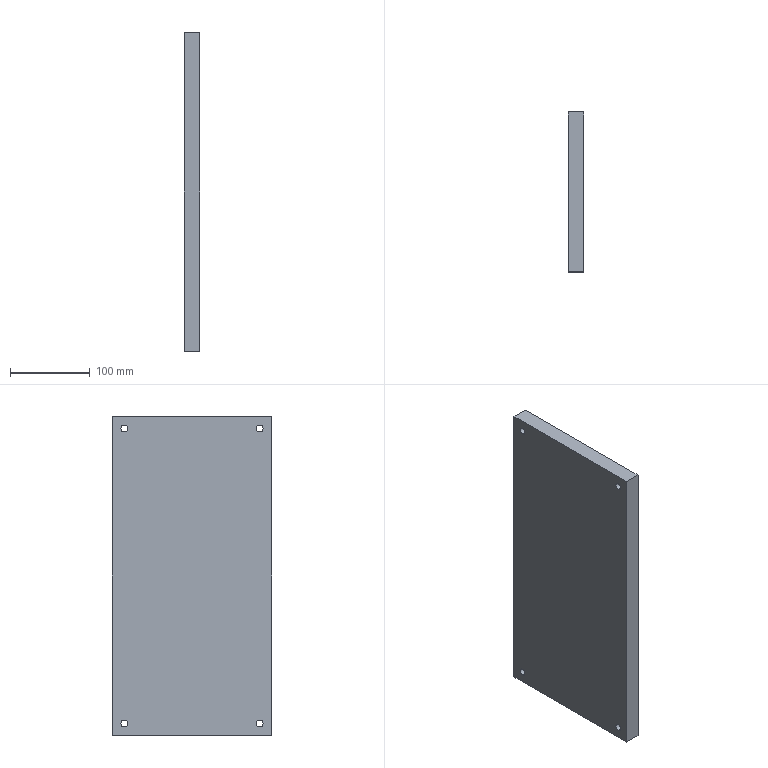Part | STEP file | A14-030-1 | 1 solid | 14 faces | box 20 x 200 x 400 mm | volume 1595460 mm3 | cylinder 8 | plane 6 | commonest cylinder face diameters 8.5 x8
STEP:
#1=CARTESIAN_POINT('',(0.,0.,0.));
#2=DIRECTION('',(0.,0.,1.));
#3=DIRECTION('',(1.,0.,0.));
#4=AXIS2_PLACEMENT_3D('',#1,#2,#3);
#5=CARTESIAN_POINT('',(-10.,85.,180.75));
#6=VERTEX_POINT('',#5);
#7=CARTESIAN_POINT('',(10.,85.,180.75));
#8=VERTEX_POINT('',#7);
#9=CARTESIAN_POINT('',(-10.,85.,180.75));
#10=DIRECTION('',(1.,0.,0.));
#11=VECTOR('',#10,1.);
#12=LINE('',#9,#11);
#13=CARTESIAN_POINT('',(-10.,85.,185.));
#14=DIRECTION('',(1.,0.,0.));
#15=DIRECTION('',(0.,0.,-1.));
#16=AXIS2_PLACEMENT_3D('',#13,#14,#15);
#17=CYLINDRICAL_SURFACE('',#16,4.25);
#18=CARTESIAN_POINT('',(6.283,0.));
#19=DIRECTION('',(0.,1.));
#20=VECTOR('',#19,1.);
#21=LINE('',#18,#20);
#22=(GEOMETRIC_REPRESENTATION_CONTEXT(2)PARAMETRIC_REPRESENTATION_CONTEXT()REPRESENTATION_CONTEXT('',''));
#23=DEFINITIONAL_REPRESENTATION('',(#21),#22);
#24=PCURVE('',#17,#23);
#25=CARTESIAN_POINT('',(-10.,85.,185.));
#26=DIRECTION('',(1.,0.,0.));
#27=DIRECTION('',(0.,0.,-1.));
#28=AXIS2_PLACEMENT_3D('',#25,#26,#27);
#29=CYLINDRICAL_SURFACE('',#28,4.25);
#30=CARTESIAN_POINT('',(0.,0.));
#31=DIRECTION('',(0.,1.));
#32=VECTOR('',#31,1.);
#33=LINE('',#30,#32);
#34=(GEOMETRIC_REPRESENTATION_CONTEXT(2)PARAMETRIC_REPRESENTATION_CONTEXT()REPRESENTATION_CONTEXT('',''));
#35=DEFINITIONAL_REPRESENTATION('',(#33),#34);
#36=PCURVE('',#29,#35);
#37=SURFACE_CURVE('',#12,(#24,#36),.PCURVE_S1.);
#38=EDGE_CURVE('',#6,#8,#37,.T.);
#39=ORIENTED_EDGE('',*,*,#38,.T.);
#40=CARTESIAN_POINT('',(10.,85.,189.25));
#41=VERTEX_POINT('',#40);
#42=CARTESIAN_POINT('',(10.,85.,185.));
#43=DIRECTION('',(1.,0.,0.));
#44=DIRECTION('',(0.,0.,-1.));
#45=AXIS2_PLACEMENT_3D('',#42,#43,#44);
#46=CIRCLE('',#45,4.25);
#47=CARTESIAN_POINT('',(0.,20.));
#48=DIRECTION('',(1.,0.));
#49=VECTOR('',#48,1.);
#50=LINE('',#47,#49);
#51=(GEOMETRIC_REPRESENTATION_CONTEXT(2)PARAMETRIC_REPRESENTATION_CONTEXT()REPRESENTATION_CONTEXT('',''));
#52=DEFINITIONAL_REPRESENTATION('',(#50),#51);
#53=PCURVE('',#17,#52);
#54=CARTESIAN_POINT('',(10.,0.,0.));
#55=DIRECTION('',(1.,0.,0.));
#56=DIRECTION('',(0.,0.,-1.));
#57=AXIS2_PLACEMENT_3D('',#54,#55,#56);
#58=PLANE('',#57);
#59=CARTESIAN_POINT('',(-185.,85.));
#60=DIRECTION('',(1.,0.));
#61=AXIS2_PLACEMENT_2D('',#59,#60);
#62=CIRCLE('',#61,4.25);
#63=(GEOMETRIC_REPRESENTATION_CONTEXT(2)PARAMETRIC_REPRESENTATION_CONTEXT()REPRESENTATION_CONTEXT('',''));
#64=DEFINITIONAL_REPRESENTATION('',(#62),#63);
#65=PCURVE('',#58,#64);
#66=SURFACE_CURVE('',#46,(#53,#65),.PCURVE_S1.);
#67=EDGE_CURVE('',#41,#8,#66,.T.);
#68=ORIENTED_EDGE('',*,*,#67,.F.);
#69=CARTESIAN_POINT('',(-10.,85.,189.25));
#70=VERTEX_POINT('',#69);
#71=CARTESIAN_POINT('',(-10.,85.,189.25));
#72=DIRECTION('',(1.,0.,0.));
#73=VECTOR('',#72,1.);
#74=LINE('',#71,#73);
#75=CARTESIAN_POINT('',(3.142,0.));
#76=DIRECTION('',(0.,1.));
#77=VECTOR('',#76,1.);
#78=LINE('',#75,#77);
#79=(GEOMETRIC_REPRESENTATION_CONTEXT(2)PARAMETRIC_REPRESENTATION_CONTEXT()REPRESENTATION_CONTEXT('',''));
#80=DEFINITIONAL_REPRESENTATION('',(#78),#79);
#81=PCURVE('',#17,#80);
#82=CARTESIAN_POINT('',(3.142,0.));
#83=DIRECTION('',(0.,1.));
#84=VECTOR('',#83,1.);
#85=LINE('',#82,#84);
#86=(GEOMETRIC_REPRESENTATION_CONTEXT(2)PARAMETRIC_REPRESENTATION_CONTEXT()REPRESENTATION_CONTEXT('',''));
#87=DEFINITIONAL_REPRESENTATION('',(#85),#86);
#88=PCURVE('',#29,#87);
#89=SURFACE_CURVE('',#74,(#81,#88),.PCURVE_S1.);
#90=EDGE_CURVE('',#70,#41,#89,.T.);
#91=ORIENTED_EDGE('',*,*,#90,.F.);
#92=CARTESIAN_POINT('',(-10.,85.,185.));
#93=DIRECTION('',(1.,0.,0.));
#94=DIRECTION('',(0.,0.,-1.));
#95=AXIS2_PLACEMENT_3D('',#92,#93,#94);
#96=CIRCLE('',#95,4.25);
#97=CARTESIAN_POINT('',(0.,0.));
#98=DIRECTION('',(1.,0.));
#99=VECTOR('',#98,1.);
#100=LINE('',#97,#99);
#101=(GEOMETRIC_REPRESENTATION_CONTEXT(2)PARAMETRIC_REPRESENTATION_CONTEXT()REPRESENTATION_CONTEXT('',''));
#102=DEFINITIONAL_REPRESENTATION('',(#100),#101);
#103=PCURVE('',#17,#102);
#104=CARTESIAN_POINT('',(-10.,0.,0.));
#105=DIRECTION('',(1.,0.,0.));
#106=DIRECTION('',(0.,0.,-1.));
#107=AXIS2_PLACEMENT_3D('',#104,#105,#106);
#108=PLANE('',#107);
#109=CARTESIAN_POINT('',(-185.,85.));
#110=DIRECTION('',(1.,0.));
#111=AXIS2_PLACEMENT_2D('',#109,#110);
#112=CIRCLE('',#111,4.25);
#113=(GEOMETRIC_REPRESENTATION_CONTEXT(2)PARAMETRIC_REPRESENTATION_CONTEXT()REPRESENTATION_CONTEXT('',''));
#114=DEFINITIONAL_REPRESENTATION('',(#112),#113);
#115=PCURVE('',#108,#114);
#116=SURFACE_CURVE('',#96,(#103,#115),.PCURVE_S1.);
#117=EDGE_CURVE('',#70,#6,#116,.T.);
#118=ORIENTED_EDGE('',*,*,#117,.T.);
#119=EDGE_LOOP('',(#39,#68,#91,#118));
#120=FACE_BOUND('',#119,.F.);
#121=ADVANCED_FACE('',(#120),#17,.F.);
#122=CARTESIAN_POINT('',(-10.,-85.,180.75));
#123=VERTEX_POINT('',#122);
#124=CARTESIAN_POINT('',(10.,-85.,180.75));
#125=VERTEX_POINT('',#124);
#126=CARTESIAN_POINT('',(-10.,-85.,180.75));
#127=DIRECTION('',(1.,0.,0.));
#128=VECTOR('',#127,1.);
#129=LINE('',#126,#128);
#130=CARTESIAN_POINT('',(-10.,-85.,185.));
#131=DIRECTION('',(1.,0.,0.));
#132=DIRECTION('',(0.,0.,-1.));
#133=AXIS2_PLACEMENT_3D('',#130,#131,#132);
#134=CYLINDRICAL_SURFACE('',#133,4.25);
#135=CARTESIAN_POINT('',(6.283,0.));
#136=DIRECTION('',(0.,1.));
#137=VECTOR('',#136,1.);
#138=LINE('',#135,#137);
#139=(GEOMETRIC_REPRESENTATION_CONTEXT(2)PARAMETRIC_REPRESENTATION_CONTEXT()REPRESENTATION_CONTEXT('',''));
#140=DEFINITIONAL_REPRESENTATION('',(#138),#139);
#141=PCURVE('',#134,#140);
#142=CARTESIAN_POINT('',(-10.,-85.,185.));
#143=DIRECTION('',(1.,0.,0.));
#144=DIRECTION('',(0.,0.,-1.));
#145=AXIS2_PLACEMENT_3D('',#142,#143,#144);
#146=CYLINDRICAL_SURFACE('',#145,4.25);
#147=CARTESIAN_POINT('',(0.,0.));
#148=DIRECTION('',(0.,1.));
#149=VECTOR('',#148,1.);
#150=LINE('',#147,#149);
#151=(GEOMETRIC_REPRESENTATION_CONTEXT(2)PARAMETRIC_REPRESENTATION_CONTEXT()REPRESENTATION_CONTEXT('',''));
#152=DEFINITIONAL_REPRESENTATION('',(#150),#151);
#153=PCURVE('',#146,#152);
#154=SURFACE_CURVE('',#129,(#141,#153),.PCURVE_S1.);
#155=EDGE_CURVE('',#123,#125,#154,.T.);
#156=ORIENTED_EDGE('',*,*,#155,.T.);
#157=CARTESIAN_POINT('',(10.,-85.,189.25));
#158=VERTEX_POINT('',#157);
#159=CARTESIAN_POINT('',(10.,-85.,185.));
#160=DIRECTION('',(1.,0.,0.));
#161=DIRECTION('',(0.,0.,-1.));
#162=AXIS2_PLACEMENT_3D('',#159,#160,#161);
#163=CIRCLE('',#162,4.25);
#164=CARTESIAN_POINT('',(0.,20.));
#165=DIRECTION('',(1.,0.));
#166=VECTOR('',#165,1.);
#167=LINE('',#164,#166);
#168=(GEOMETRIC_REPRESENTATION_CONTEXT(2)PARAMETRIC_REPRESENTATION_CONTEXT()REPRESENTATION_CONTEXT('',''));
#169=DEFINITIONAL_REPRESENTATION('',(#167),#168);
#170=PCURVE('',#134,#169);
#171=CARTESIAN_POINT('',(-185.,-85.));
#172=DIRECTION('',(1.,0.));
#173=AXIS2_PLACEMENT_2D('',#171,#172);
#174=CIRCLE('',#173,4.25);
#175=(GEOMETRIC_REPRESENTATION_CONTEXT(2)PARAMETRIC_REPRESENTATION_CONTEXT()REPRESENTATION_CONTEXT('',''));
#176=DEFINITIONAL_REPRESENTATION('',(#174),#175);
#177=PCURVE('',#58,#176);
#178=SURFACE_CURVE('',#163,(#170,#177),.PCURVE_S1.);
#179=EDGE_CURVE('',#158,#125,#178,.T.);
#180=ORIENTED_EDGE('',*,*,#179,.F.);
#181=CARTESIAN_POINT('',(-10.,-85.,189.25));
#182=VERTEX_POINT('',#181);
#183=CARTESIAN_POINT('',(-10.,-85.,189.25));
#184=DIRECTION('',(1.,0.,0.));
#185=VECTOR('',#184,1.);
#186=LINE('',#183,#185);
#187=CARTESIAN_POINT('',(3.142,0.));
#188=DIRECTION('',(0.,1.));
#189=VECTOR('',#188,1.);
#190=LINE('',#187,#189);
#191=(GEOMETRIC_REPRESENTATION_CONTEXT(2)PARAMETRIC_REPRESENTATION_CONTEXT()REPRESENTATION_CONTEXT('',''));
#192=DEFINITIONAL_REPRESENTATION('',(#190),#191);
#193=PCURVE('',#134,#192);
#194=CARTESIAN_POINT('',(3.142,0.));
#195=DIRECTION('',(0.,1.));
#196=VECTOR('',#195,1.);
#197=LINE('',#194,#196);
#198=(GEOMETRIC_REPRESENTATION_CONTEXT(2)PARAMETRIC_REPRESENTATION_CONTEXT()REPRESENTATION_CONTEXT('',''));
#199=DEFINITIONAL_REPRESENTATION('',(#197),#198);
#200=PCURVE('',#146,#199);
#201=SURFACE_CURVE('',#186,(#193,#200),.PCURVE_S1.);
#202=EDGE_CURVE('',#182,#158,#201,.T.);
#203=ORIENTED_EDGE('',*,*,#202,.F.);
#204=CARTESIAN_POINT('',(-10.,-85.,185.));
#205=DIRECTION('',(1.,0.,0.));
#206=DIRECTION('',(0.,0.,-1.));
#207=AXIS2_PLACEMENT_3D('',#204,#205,#206);
#208=CIRCLE('',#207,4.25);
#209=CARTESIAN_POINT('',(0.,0.));
#210=DIRECTION('',(1.,0.));
#211=VECTOR('',#210,1.);
#212=LINE('',#209,#211);
#213=(GEOMETRIC_REPRESENTATION_CONTEXT(2)PARAMETRIC_REPRESENTATION_CONTEXT()REPRESENTATION_CONTEXT('',''));
#214=DEFINITIONAL_REPRESENTATION('',(#212),#213);
#215=PCURVE('',#134,#214);
#216=CARTESIAN_POINT('',(-185.,-85.));
#217=DIRECTION('',(1.,0.));
#218=AXIS2_PLACEMENT_2D('',#216,#217);
#219=CIRCLE('',#218,4.25);
#220=(GEOMETRIC_REPRESENTATION_CONTEXT(2)PARAMETRIC_REPRESENTATION_CONTEXT()REPRESENTATION_CONTEXT('',''));
#221=DEFINITIONAL_REPRESENTATION('',(#219),#220);
#222=PCURVE('',#108,#221);
#223=SURFACE_CURVE('',#208,(#215,#222),.PCURVE_S1.);
#224=EDGE_CURVE('',#182,#123,#223,.T.);
#225=ORIENTED_EDGE('',*,*,#224,.T.);
#226=EDGE_LOOP('',(#156,#180,#203,#225));
#227=FACE_BOUND('',#226,.F.);
#228=ADVANCED_FACE('',(#227),#134,.F.);
#229=CARTESIAN_POINT('',(-10.,-85.,-189.25));
#230=VERTEX_POINT('',#229);
#231=CARTESIAN_POINT('',(10.,-85.,-189.25));
#232=VERTEX_POINT('',#231);
#233=CARTESIAN_POINT('',(-10.,-85.,-189.25));
#234=DIRECTION('',(1.,0.,0.));
#235=VECTOR('',#234,1.);
#236=LINE('',#233,#235);
#237=CARTESIAN_POINT('',(-10.,-85.,-185.));
#238=DIRECTION('',(1.,0.,0.));
#239=DIRECTION('',(0.,0.,-1.));
#240=AXIS2_PLACEMENT_3D('',#237,#238,#239);
#241=CYLINDRICAL_SURFACE('',#240,4.25);
#242=CARTESIAN_POINT('',(6.283,0.));
#243=DIRECTION('',(0.,1.));
#244=VECTOR('',#243,1.);
#245=LINE('',#242,#244);
#246=(GEOMETRIC_REPRESENTATION_CONTEXT(2)PARAMETRIC_REPRESENTATION_CONTEXT()REPRESENTATION_CONTEXT('',''));
#247=DEFINITIONAL_REPRESENTATION('',(#245),#246);
#248=PCURVE('',#241,#247);
#249=CARTESIAN_POINT('',(-10.,-85.,-185.));
#250=DIRECTION('',(1.,0.,0.));
#251=DIRECTION('',(0.,0.,-1.));
#252=AXIS2_PLACEMENT_3D('',#249,#250,#251);
#253=CYLINDRICAL_SURFACE('',#252,4.25);
#254=CARTESIAN_POINT('',(0.,0.));
#255=DIRECTION('',(0.,1.));
#256=VECTOR('',#255,1.);
#257=LINE('',#254,#256);
#258=(GEOMETRIC_REPRESENTATION_CONTEXT(2)PARAMETRIC_REPRESENTATION_CONTEXT()REPRESENTATION_CONTEXT('',''));
#259=DEFINITIONAL_REPRESENTATION('',(#257),#258);
#260=PCURVE('',#253,#259);
#261=SURFACE_CURVE('',#236,(#248,#260),.PCURVE_S1.);
#262=EDGE_CURVE('',#230,#232,#261,.T.);
#263=ORIENTED_EDGE('',*,*,#262,.T.);
#264=CARTESIAN_POINT('',(10.,-85.,-180.75));
#265=VERTEX_POINT('',#264);
#266=CARTESIAN_POINT('',(10.,-85.,-185.));
#267=DIRECTION('',(1.,0.,0.));
#268=DIRECTION('',(0.,0.,-1.));
#269=AXIS2_PLACEMENT_3D('',#266,#267,#268);
#270=CIRCLE('',#269,4.25);
#271=CARTESIAN_POINT('',(0.,20.));
#272=DIRECTION('',(1.,0.));
#273=VECTOR('',#272,1.);
#274=LINE('',#271,#273);
#275=(GEOMETRIC_REPRESENTATION_CONTEXT(2)PARAMETRIC_REPRESENTATION_CONTEXT()REPRESENTATION_CONTEXT('',''));
#276=DEFINITIONAL_REPRESENTATION('',(#274),#275);
#277=PCURVE('',#241,#276);
#278=CARTESIAN_POINT('',(185.,-85.));
#279=DIRECTION('',(1.,0.));
#280=AXIS2_PLACEMENT_2D('',#278,#279);
#281=CIRCLE('',#280,4.25);
#282=(GEOMETRIC_REPRESENTATION_CONTEXT(2)PARAMETRIC_REPRESENTATION_CONTEXT()REPRESENTATION_CONTEXT('',''));
#283=DEFINITIONAL_REPRESENTATION('',(#281),#282);
#284=PCURVE('',#58,#283);
#285=SURFACE_CURVE('',#270,(#277,#284),.PCURVE_S1.);
#286=EDGE_CURVE('',#265,#232,#285,.T.);
#287=ORIENTED_EDGE('',*,*,#286,.F.);
#288=CARTESIAN_POINT('',(-10.,-85.,-180.75));
#289=VERTEX_POINT('',#288);
#290=CARTESIAN_POINT('',(-10.,-85.,-180.75));
#291=DIRECTION('',(1.,0.,0.));
#292=VECTOR('',#291,1.);
#293=LINE('',#290,#292);
#294=CARTESIAN_POINT('',(3.142,0.));
#295=DIRECTION('',(0.,1.));
#296=VECTOR('',#295,1.);
#297=LINE('',#294,#296);
#298=(GEOMETRIC_REPRESENTATION_CONTEXT(2)PARAMETRIC_REPRESENTATION_CONTEXT()REPRESENTATION_CONTEXT('',''));
#299=DEFINITIONAL_REPRESENTATION('',(#297),#298);
#300=PCURVE('',#241,#299);
#301=CARTESIAN_POINT('',(3.142,0.));
#302=DIRECTION('',(0.,1.));
#303=VECTOR('',#302,1.);
#304=LINE('',#301,#303);
#305=(GEOMETRIC_REPRESENTATION_CONTEXT(2)PARAMETRIC_REPRESENTATION_CONTEXT()REPRESENTATION_CONTEXT('',''));
#306=DEFINITIONAL_REPRESENTATION('',(#304),#305);
#307=PCURVE('',#253,#306);
#308=SURFACE_CURVE('',#293,(#300,#307),.PCURVE_S1.);
#309=EDGE_CURVE('',#289,#265,#308,.T.);
#310=ORIENTED_EDGE('',*,*,#309,.F.);
#311=CARTESIAN_POINT('',(-10.,-85.,-185.));
#312=DIRECTION('',(1.,0.,0.));
#313=DIRECTION('',(0.,0.,-1.));
#314=AXIS2_PLACEMENT_3D('',#311,#312,#313);
#315=CIRCLE('',#314,4.25);
#316=CARTESIAN_POINT('',(0.,0.));
#317=DIRECTION('',(1.,0.));
#318=VECTOR('',#317,1.);
#319=LINE('',#316,#318);
#320=(GEOMETRIC_REPRESENTATION_CONTEXT(2)PARAMETRIC_REPRESENTATION_CONTEXT()REPRESENTATION_CONTEXT('',''));
#321=DEFINITIONAL_REPRESENTATION('',(#319),#320);
#322=PCURVE('',#241,#321);
#323=CARTESIAN_POINT('',(185.,-85.));
#324=DIRECTION('',(1.,0.));
#325=AXIS2_PLACEMENT_2D('',#323,#324);
#326=CIRCLE('',#325,4.25);
#327=(GEOMETRIC_REPRESENTATION_CONTEXT(2)PARAMETRIC_REPRESENTATION_CONTEXT()REPRESENTATION_CONTEXT('',''));
#328=DEFINITIONAL_REPRESENTATION('',(#326),#327);
#329=PCURVE('',#108,#328);
#330=SURFACE_CURVE('',#315,(#322,#329),.PCURVE_S1.);
#331=EDGE_CURVE('',#289,#230,#330,.T.);
#332=ORIENTED_EDGE('',*,*,#331,.T.);
#333=EDGE_LOOP('',(#263,#287,#310,#332));
#334=FACE_BOUND('',#333,.F.);
#335=ADVANCED_FACE('',(#334),#241,.F.);
#336=CARTESIAN_POINT('',(-10.,85.,-189.25));
#337=VERTEX_POINT('',#336);
#338=CARTESIAN_POINT('',(10.,85.,-189.25));
#339=VERTEX_POINT('',#338);
#340=CARTESIAN_POINT('',(-10.,85.,-189.25));
#341=DIRECTION('',(1.,0.,0.));
#342=VECTOR('',#341,1.);
#343=LINE('',#340,#342);
#344=CARTESIAN_POINT('',(-10.,85.,-185.));
#345=DIRECTION('',(1.,0.,0.));
#346=DIRECTION('',(0.,0.,-1.));
#347=AXIS2_PLACEMENT_3D('',#344,#345,#346);
#348=CYLINDRICAL_SURFACE('',#347,4.25);
#349=CARTESIAN_POINT('',(6.283,0.));
#350=DIRECTION('',(0.,1.));
#351=VECTOR('',#350,1.);
#352=LINE('',#349,#351);
#353=(GEOMETRIC_REPRESENTATION_CONTEXT(2)PARAMETRIC_REPRESENTATION_CONTEXT()REPRESENTATION_CONTEXT('',''));
#354=DEFINITIONAL_REPRESENTATION('',(#352),#353);
#355=PCURVE('',#348,#354);
#356=CARTESIAN_POINT('',(-10.,85.,-185.));
#357=DIRECTION('',(1.,0.,0.));
#358=DIRECTION('',(0.,0.,-1.));
#359=AXIS2_PLACEMENT_3D('',#356,#357,#358);
#360=CYLINDRICAL_SURFACE('',#359,4.25);
#361=CARTESIAN_POINT('',(0.,0.));
#362=DIRECTION('',(0.,1.));
#363=VECTOR('',#362,1.);
#364=LINE('',#361,#363);
#365=(GEOMETRIC_REPRESENTATION_CONTEXT(2)PARAMETRIC_REPRESENTATION_CONTEXT()REPRESENTATION_CONTEXT('',''));
#366=DEFINITIONAL_REPRESENTATION('',(#364),#365);
#367=PCURVE('',#360,#366);
#368=SURFACE_CURVE('',#343,(#355,#367),.PCURVE_S1.);
#369=EDGE_CURVE('',#337,#339,#368,.T.);
#370=ORIENTED_EDGE('',*,*,#369,.T.);
#371=CARTESIAN_POINT('',(10.,85.,-180.75));
#372=VERTEX_POINT('',#371);
#373=CARTESIAN_POINT('',(10.,85.,-185.));
#374=DIRECTION('',(1.,0.,0.));
#375=DIRECTION('',(0.,0.,-1.));
#376=AXIS2_PLACEMENT_3D('',#373,#374,#375);
#377=CIRCLE('',#376,4.25);
#378=CARTESIAN_POINT('',(0.,20.));
#379=DIRECTION('',(1.,0.));
#380=VECTOR('',#379,1.);
#381=LINE('',#378,#380);
#382=(GEOMETRIC_REPRESENTATION_CONTEXT(2)PARAMETRIC_REPRESENTATION_CONTEXT()REPRESENTATION_CONTEXT('',''));
#383=DEFINITIONAL_REPRESENTATION('',(#381),#382);
#384=PCURVE('',#348,#383);
#385=CARTESIAN_POINT('',(185.,85.));
#386=DIRECTION('',(1.,0.));
#387=AXIS2_PLACEMENT_2D('',#385,#386);
#388=CIRCLE('',#387,4.25);
#389=(GEOMETRIC_REPRESENTATION_CONTEXT(2)PARAMETRIC_REPRESENTATION_CONTEXT()REPRESENTATION_CONTEXT('',''));
#390=DEFINITIONAL_REPRESENTATION('',(#388),#389);
#391=PCURVE('',#58,#390);
#392=SURFACE_CURVE('',#377,(#384,#391),.PCURVE_S1.);
#393=EDGE_CURVE('',#372,#339,#392,.T.);
#394=ORIENTED_EDGE('',*,*,#393,.F.);
#395=CARTESIAN_POINT('',(-10.,85.,-180.75));
#396=VERTEX_POINT('',#395);
#397=CARTESIAN_POINT('',(-10.,85.,-180.75));
#398=DIRECTION('',(1.,0.,0.));
#399=VECTOR('',#398,1.);
#400=LINE('',#397,#399);
#401=CARTESIAN_POINT('',(3.142,0.));
#402=DIRECTION('',(0.,1.));
#403=VECTOR('',#402,1.);
#404=LINE('',#401,#403);
#405=(GEOMETRIC_REPRESENTATION_CONTEXT(2)PARAMETRIC_REPRESENTATION_CONTEXT()REPRESENTATION_CONTEXT('',''));
#406=DEFINITIONAL_REPRESENTATION('',(#404),#405);
#407=PCURVE('',#348,#406);
#408=CARTESIAN_POINT('',(3.142,0.));
#409=DIRECTION('',(0.,1.));
#410=VECTOR('',#409,1.);
#411=LINE('',#408,#410);
#412=(GEOMETRIC_REPRESENTATION_CONTEXT(2)PARAMETRIC_REPRESENTATION_CONTEXT()REPRESENTATION_CONTEXT('',''));
#413=DEFINITIONAL_REPRESENTATION('',(#411),#412);
#414=PCURVE('',#360,#413);
#415=SURFACE_CURVE('',#400,(#407,#414),.PCURVE_S1.);
#416=EDGE_CURVE('',#396,#372,#415,.T.);
#417=ORIENTED_EDGE('',*,*,#416,.F.);
#418=CARTESIAN_POINT('',(-10.,85.,-185.));
#419=DIRECTION('',(1.,0.,0.));
#420=DIRECTION('',(0.,0.,-1.));
#421=AXIS2_PLACEMENT_3D('',#418,#419,#420);
#422=CIRCLE('',#421,4.25);
#423=CARTESIAN_POINT('',(0.,0.));
#424=DIRECTION('',(1.,0.));
#425=VECTOR('',#424,1.);
#426=LINE('',#423,#425);
#427=(GEOMETRIC_REPRESENTATION_CONTEXT(2)PARAMETRIC_REPRESENTATION_CONTEXT()REPRESENTATION_CONTEXT('',''));
#428=DEFINITIONAL_REPRESENTATION('',(#426),#427);
#429=PCURVE('',#348,#428);
#430=CARTESIAN_POINT('',(185.,85.));
#431=DIRECTION('',(1.,0.));
#432=AXIS2_PLACEMENT_2D('',#430,#431);
#433=CIRCLE('',#432,4.25);
#434=(GEOMETRIC_REPRESENTATION_CONTEXT(2)PARAMETRIC_REPRESENTATION_CONTEXT()REPRESENTATION_CONTEXT('',''));
#435=DEFINITIONAL_REPRESENTATION('',(#433),#434);
#436=PCURVE('',#108,#435);
#437=SURFACE_CURVE('',#422,(#429,#436),.PCURVE_S1.);
#438=EDGE_CURVE('',#396,#337,#437,.T.);
#439=ORIENTED_EDGE('',*,*,#438,.T.);
#440=EDGE_LOOP('',(#370,#394,#417,#439));
#441=FACE_BOUND('',#440,.F.);
#442=ADVANCED_FACE('',(#441),#348,.F.);
#443=CARTESIAN_POINT('',(-10.,-100.,-200.));
#444=VERTEX_POINT('',#443);
#445=CARTESIAN_POINT('',(-10.,100.,-200.));
#446=VERTEX_POINT('',#445);
#447=CARTESIAN_POINT('',(-10.,100.,-200.));
#448=DIRECTION('',(0.,1.,0.));
#449=VECTOR('',#448,1.);
#450=LINE('',#447,#449);
#451=CARTESIAN_POINT('',(10.,100.,-200.));
#452=DIRECTION('',(0.,0.,1.));
#453=DIRECTION('',(0.,-1.,0.));
#454=AXIS2_PLACEMENT_3D('',#451,#452,#453);
#455=PLANE('',#454);
#456=CARTESIAN_POINT('',(0.,-20.));
#457=DIRECTION('',(-1.,0.));
#458=VECTOR('',#457,1.);
#459=LINE('',#456,#458);
#460=(GEOMETRIC_REPRESENTATION_CONTEXT(2)PARAMETRIC_REPRESENTATION_CONTEXT()REPRESENTATION_CONTEXT('',''));
#461=DEFINITIONAL_REPRESENTATION('',(#459),#460);
#462=PCURVE('',#455,#461);
#463=CARTESIAN_POINT('',(200.,100.));
#464=DIRECTION('',(0.,1.));
#465=VECTOR('',#464,1.);
#466=LINE('',#463,#465);
#467=(GEOMETRIC_REPRESENTATION_CONTEXT(2)PARAMETRIC_REPRESENTATION_CONTEXT()REPRESENTATION_CONTEXT('',''));
#468=DEFINITIONAL_REPRESENTATION('',(#466),#467);
#469=PCURVE('',#108,#468);
#470=SURFACE_CURVE('',#450,(#462,#469),.PCURVE_S1.);
#471=EDGE_CURVE('',#444,#446,#470,.T.);
#472=ORIENTED_EDGE('',*,*,#471,.T.);
#473=CARTESIAN_POINT('',(10.,100.,-200.));
#474=VERTEX_POINT('',#473);
#475=CARTESIAN_POINT('',(10.,100.,-200.));
#476=DIRECTION('',(-1.,0.,0.));
#477=VECTOR('',#476,1.);
#478=LINE('',#475,#477);
#479=CARTESIAN_POINT('',(0.,0.));
#480=DIRECTION('',(0.,-1.));
#481=VECTOR('',#480,1.);
#482=LINE('',#479,#481);
#483=(GEOMETRIC_REPRESENTATION_CONTEXT(2)PARAMETRIC_REPRESENTATION_CONTEXT()REPRESENTATION_CONTEXT('',''));
#484=DEFINITIONAL_REPRESENTATION('',(#482),#483);
#485=PCURVE('',#455,#484);
#486=CARTESIAN_POINT('',(10.,100.,200.));
#487=DIRECTION('',(0.,-1.,0.));
#488=DIRECTION('',(0.,0.,-1.));
#489=AXIS2_PLACEMENT_3D('',#486,#487,#488);
#490=PLANE('',#489);
#491=CARTESIAN_POINT('',(400.,0.));
#492=DIRECTION('',(0.,-1.));
#493=VECTOR('',#492,1.);
#494=LINE('',#491,#493);
#495=(GEOMETRIC_REPRESENTATION_CONTEXT(2)PARAMETRIC_REPRESENTATION_CONTEXT()REPRESENTATION_CONTEXT('',''));
#496=DEFINITIONAL_REPRESENTATION('',(#494),#495);
#497=PCURVE('',#490,#496);
#498=SURFACE_CURVE('',#478,(#485,#497),.PCURVE_S1.);
#499=EDGE_CURVE('',#474,#446,#498,.T.);
#500=ORIENTED_EDGE('',*,*,#499,.F.);
#501=CARTESIAN_POINT('',(10.,-100.,-200.));
#502=VERTEX_POINT('',#501);
#503=CARTESIAN_POINT('',(10.,100.,-200.));
#504=DIRECTION('',(0.,1.,0.));
#505=VECTOR('',#504,1.);
#506=LINE('',#503,#505);
#507=CARTESIAN_POINT('',(0.,0.));
#508=DIRECTION('',(-1.,0.));
#509=VECTOR('',#508,1.);
#510=LINE('',#507,#509);
#511=(GEOMETRIC_REPRESENTATION_CONTEXT(2)PARAMETRIC_REPRESENTATION_CONTEXT()REPRESENTATION_CONTEXT('',''));
#512=DEFINITIONAL_REPRESENTATION('',(#510),#511);
#513=PCURVE('',#455,#512);
#514=CARTESIAN_POINT('',(200.,100.));
#515=DIRECTION('',(0.,1.));
#516=VECTOR('',#515,1.);
#517=LINE('',#514,#516);
#518=(GEOMETRIC_REPRESENTATION_CONTEXT(2)PARAMETRIC_REPRESENTATION_CONTEXT()REPRESENTATION_CONTEXT('',''));
#519=DEFINITIONAL_REPRESENTATION('',(#517),#518);
#520=PCURVE('',#58,#519);
#521=SURFACE_CURVE('',#506,(#513,#520),.PCURVE_S1.);
#522=EDGE_CURVE('',#502,#474,#521,.T.);
#523=ORIENTED_EDGE('',*,*,#522,.F.);
#524=CARTESIAN_POINT('',(10.,-100.,-200.));
#525=DIRECTION('',(-1.,0.,0.));
#526=VECTOR('',#525,1.);
#527=LINE('',#524,#526);
#528=CARTESIAN_POINT('',(200.,0.));
#529=DIRECTION('',(0.,-1.));
#530=VECTOR('',#529,1.);
#531=LINE('',#528,#530);
#532=(GEOMETRIC_REPRESENTATION_CONTEXT(2)PARAMETRIC_REPRESENTATION_CONTEXT()REPRESENTATION_CONTEXT('',''));
#533=DEFINITIONAL_REPRESENTATION('',(#531),#532);
#534=PCURVE('',#455,#533);
#535=CARTESIAN_POINT('',(10.,-100.,200.));
#536=DIRECTION('',(0.,1.,0.));
#537=DIRECTION('',(0.,0.,1.));
#538=AXIS2_PLACEMENT_3D('',#535,#536,#537);
#539=PLANE('',#538);
#540=CARTESIAN_POINT('',(-400.,0.));
#541=DIRECTION('',(0.,-1.));
#542=VECTOR('',#541,1.);
#543=LINE('',#540,#542);
#544=(GEOMETRIC_REPRESENTATION_CONTEXT(2)PARAMETRIC_REPRESENTATION_CONTEXT()REPRESENTATION_CONTEXT('',''));
#545=DEFINITIONAL_REPRESENTATION('',(#543),#544);
#546=PCURVE('',#539,#545);
#547=SURFACE_CURVE('',#527,(#534,#546),.PCURVE_S1.);
#548=EDGE_CURVE('',#502,#444,#547,.T.);
#549=ORIENTED_EDGE('',*,*,#548,.T.);
#550=EDGE_LOOP('',(#472,#500,#523,#549));
#551=FACE_BOUND('',#550,.T.);
#552=ADVANCED_FACE('',(#551),#455,.F.);
#553=CARTESIAN_POINT('',(-10.,100.,200.));
#554=VERTEX_POINT('',#553);
#555=CARTESIAN_POINT('',(-10.,100.,200.));
#556=DIRECTION('',(0.,0.,1.));
#557=VECTOR('',#556,1.);
#558=LINE('',#555,#557);
#559=CARTESIAN_POINT('',(0.,-20.));
#560=DIRECTION('',(-1.,0.));
#561=VECTOR('',#560,1.);
#562=LINE('',#559,#561);
#563=(GEOMETRIC_REPRESENTATION_CONTEXT(2)PARAMETRIC_REPRESENTATION_CONTEXT()REPRESENTATION_CONTEXT('',''));
#564=DEFINITIONAL_REPRESENTATION('',(#562),#563);
#565=PCURVE('',#490,#564);
#566=CARTESIAN_POINT('',(-200.,100.));
#567=DIRECTION('',(-1.,0.));
#568=VECTOR('',#567,1.);
#569=LINE('',#566,#568);
#570=(GEOMETRIC_REPRESENTATION_CONTEXT(2)PARAMETRIC_REPRESENTATION_CONTEXT()REPRESENTATION_CONTEXT('',''));
#571=DEFINITIONAL_REPRESENTATION('',(#569),#570);
#572=PCURVE('',#108,#571);
#573=SURFACE_CURVE('',#558,(#565,#572),.PCURVE_S1.);
#574=EDGE_CURVE('',#446,#554,#573,.T.);
#575=ORIENTED_EDGE('',*,*,#574,.T.);
#576=CARTESIAN_POINT('',(10.,100.,200.));
#577=VERTEX_POINT('',#576);
#578=CARTESIAN_POINT('',(10.,100.,200.));
#579=DIRECTION('',(-1.,0.,0.));
#580=VECTOR('',#579,1.);
#581=LINE('',#578,#580);
#582=CARTESIAN_POINT('',(0.,0.));
#583=DIRECTION('',(0.,-1.));
#584=VECTOR('',#583,1.);
#585=LINE('',#582,#584);
#586=(GEOMETRIC_REPRESENTATION_CONTEXT(2)PARAMETRIC_REPRESENTATION_CONTEXT()REPRESENTATION_CONTEXT('',''));
#587=DEFINITIONAL_REPRESENTATION('',(#585),#586);
#588=PCURVE('',#490,#587);
#589=CARTESIAN_POINT('',(10.,100.,200.));
#590=DIRECTION('',(0.,0.,-1.));
#591=DIRECTION('',(0.,1.,0.));
#592=AXIS2_PLACEMENT_3D('',#589,#590,#591);
#593=PLANE('',#592);
#594=CARTESIAN_POINT('',(0.,0.));
#595=DIRECTION('',(0.,-1.));
#596=VECTOR('',#595,1.);
#597=LINE('',#594,#596);
#598=(GEOMETRIC_REPRESENTATION_CONTEXT(2)PARAMETRIC_REPRESENTATION_CONTEXT()REPRESENTATION_CONTEXT('',''));
#599=DEFINITIONAL_REPRESENTATION('',(#597),#598);
#600=PCURVE('',#593,#599);
#601=SURFACE_CURVE('',#581,(#588,#600),.PCURVE_S1.);
#602=EDGE_CURVE('',#577,#554,#601,.T.);
#603=ORIENTED_EDGE('',*,*,#602,.F.);
#604=CARTESIAN_POINT('',(10.,100.,200.));
#605=DIRECTION('',(0.,0.,1.));
#606=VECTOR('',#605,1.);
#607=LINE('',#604,#606);
#608=CARTESIAN_POINT('',(0.,0.));
#609=DIRECTION('',(-1.,0.));
#610=VECTOR('',#609,1.);
#611=LINE('',#608,#610);
#612=(GEOMETRIC_REPRESENTATION_CONTEXT(2)PARAMETRIC_REPRESENTATION_CONTEXT()REPRESENTATION_CONTEXT('',''));
#613=DEFINITIONAL_REPRESENTATION('',(#611),#612);
#614=PCURVE('',#490,#613);
#615=CARTESIAN_POINT('',(-200.,100.));
#616=DIRECTION('',(-1.,0.));
#617=VECTOR('',#616,1.);
#618=LINE('',#615,#617);
#619=(GEOMETRIC_REPRESENTATION_CONTEXT(2)PARAMETRIC_REPRESENTATION_CONTEXT()REPRESENTATION_CONTEXT('',''));
#620=DEFINITIONAL_REPRESENTATION('',(#618),#619);
#621=PCURVE('',#58,#620);
#622=SURFACE_CURVE('',#607,(#614,#621),.PCURVE_S1.);
#623=EDGE_CURVE('',#474,#577,#622,.T.);
#624=ORIENTED_EDGE('',*,*,#623,.F.);
#625=ORIENTED_EDGE('',*,*,#499,.T.);
#626=EDGE_LOOP('',(#575,#603,#624,#625));
#627=FACE_BOUND('',#626,.T.);
#628=ADVANCED_FACE('',(#627),#490,.F.);
#629=CARTESIAN_POINT('',(-10.,-100.,200.));
#630=VERTEX_POINT('',#629);
#631=CARTESIAN_POINT('',(-10.,100.,200.));
#632=DIRECTION('',(0.,-1.,0.));
#633=VECTOR('',#632,1.);
#634=LINE('',#631,#633);
#635=CARTESIAN_POINT('',(0.,-20.));
#636=DIRECTION('',(-1.,0.));
#637=VECTOR('',#636,1.);
#638=LINE('',#635,#637);
#639=(GEOMETRIC_REPRESENTATION_CONTEXT(2)PARAMETRIC_REPRESENTATION_CONTEXT()REPRESENTATION_CONTEXT('',''));
#640=DEFINITIONAL_REPRESENTATION('',(#638),#639);
#641=PCURVE('',#593,#640);
#642=CARTESIAN_POINT('',(-200.,100.));
#643=DIRECTION('',(0.,-1.));
#644=VECTOR('',#643,1.);
#645=LINE('',#642,#644);
#646=(GEOMETRIC_REPRESENTATION_CONTEXT(2)PARAMETRIC_REPRESENTATION_CONTEXT()REPRESENTATION_CONTEXT('',''));
#647=DEFINITIONAL_REPRESENTATION('',(#645),#646);
#648=PCURVE('',#108,#647);
#649=SURFACE_CURVE('',#634,(#641,#648),.PCURVE_S1.);
#650=EDGE_CURVE('',#554,#630,#649,.T.);
#651=ORIENTED_EDGE('',*,*,#650,.T.);
#652=CARTESIAN_POINT('',(10.,-100.,200.));
#653=VERTEX_POINT('',#652);
#654=CARTESIAN_POINT('',(10.,-100.,200.));
#655=DIRECTION('',(-1.,0.,0.));
#656=VECTOR('',#655,1.);
#657=LINE('',#654,#656);
#658=CARTESIAN_POINT('',(-200.,0.));
#659=DIRECTION('',(0.,-1.));
#660=VECTOR('',#659,1.);
#661=LINE('',#658,#660);
#662=(GEOMETRIC_REPRESENTATION_CONTEXT(2)PARAMETRIC_REPRESENTATION_CONTEXT()REPRESENTATION_CONTEXT('',''));
#663=DEFINITIONAL_REPRESENTATION('',(#661),#662);
#664=PCURVE('',#593,#663);
#665=CARTESIAN_POINT('',(0.,0.));
#666=DIRECTION('',(0.,-1.));
#667=VECTOR('',#666,1.);
#668=LINE('',#665,#667);
#669=(GEOMETRIC_REPRESENTATION_CONTEXT(2)PARAMETRIC_REPRESENTATION_CONTEXT()REPRESENTATION_CONTEXT('',''));
#670=DEFINITIONAL_REPRESENTATION('',(#668),#669);
#671=PCURVE('',#539,#670);
#672=SURFACE_CURVE('',#657,(#664,#671),.PCURVE_S1.);
#673=EDGE_CURVE('',#653,#630,#672,.T.);
#674=ORIENTED_EDGE('',*,*,#673,.F.);
#675=CARTESIAN_POINT('',(10.,100.,200.));
#676=DIRECTION('',(0.,-1.,0.));
#677=VECTOR('',#676,1.);
#678=LINE('',#675,#677);
#679=CARTESIAN_POINT('',(0.,0.));
#680=DIRECTION('',(-1.,0.));
#681=VECTOR('',#680,1.);
#682=LINE('',#679,#681);
#683=(GEOMETRIC_REPRESENTATION_CONTEXT(2)PARAMETRIC_REPRESENTATION_CONTEXT()REPRESENTATION_CONTEXT('',''));
#684=DEFINITIONAL_REPRESENTATION('',(#682),#683);
#685=PCURVE('',#593,#684);
#686=CARTESIAN_POINT('',(-200.,100.));
#687=DIRECTION('',(0.,-1.));
#688=VECTOR('',#687,1.);
#689=LINE('',#686,#688);
#690=(GEOMETRIC_REPRESENTATION_CONTEXT(2)PARAMETRIC_REPRESENTATION_CONTEXT()REPRESENTATION_CONTEXT('',''));
#691=DEFINITIONAL_REPRESENTATION('',(#689),#690);
#692=PCURVE('',#58,#691);
#693=SURFACE_CURVE('',#678,(#685,#692),.PCURVE_S1.);
#694=EDGE_CURVE('',#577,#653,#693,.T.);
#695=ORIENTED_EDGE('',*,*,#694,.F.);
#696=ORIENTED_EDGE('',*,*,#602,.T.);
#697=EDGE_LOOP('',(#651,#674,#695,#696));
#698=FACE_BOUND('',#697,.T.);
#699=ADVANCED_FACE('',(#698),#593,.F.);
#700=CARTESIAN_POINT('',(-10.,-100.,200.));
#701=DIRECTION('',(0.,0.,-1.));
#702=VECTOR('',#701,1.);
#703=LINE('',#700,#702);
#704=CARTESIAN_POINT('',(0.,-20.));
#705=DIRECTION('',(-1.,0.));
#706=VECTOR('',#705,1.);
#707=LINE('',#704,#706);
#708=(GEOMETRIC_REPRESENTATION_CONTEXT(2)PARAMETRIC_REPRESENTATION_CONTEXT()REPRESENTATION_CONTEXT('',''));
#709=DEFINITIONAL_REPRESENTATION('',(#707),#708);
#710=PCURVE('',#539,#709);
#711=CARTESIAN_POINT('',(-200.,-100.));
#712=DIRECTION('',(1.,0.));
#713=VECTOR('',#712,1.);
#714=LINE('',#711,#713);
#715=(GEOMETRIC_REPRESENTATION_CONTEXT(2)PARAMETRIC_REPRESENTATION_CONTEXT()REPRESENTATION_CONTEXT('',''));
#716=DEFINITIONAL_REPRESENTATION('',(#714),#715);
#717=PCURVE('',#108,#716);
#718=SURFACE_CURVE('',#703,(#710,#717),.PCURVE_S1.);
#719=EDGE_CURVE('',#630,#444,#718,.T.);
#720=ORIENTED_EDGE('',*,*,#719,.T.);
#721=ORIENTED_EDGE('',*,*,#548,.F.);
#722=CARTESIAN_POINT('',(10.,-100.,200.));
#723=DIRECTION('',(0.,0.,-1.));
#724=VECTOR('',#723,1.);
#725=LINE('',#722,#724);
#726=CARTESIAN_POINT('',(0.,0.));
#727=DIRECTION('',(-1.,0.));
#728=VECTOR('',#727,1.);
#729=LINE('',#726,#728);
#730=(GEOMETRIC_REPRESENTATION_CONTEXT(2)PARAMETRIC_REPRESENTATION_CONTEXT()REPRESENTATION_CONTEXT('',''));
#731=DEFINITIONAL_REPRESENTATION('',(#729),#730);
#732=PCURVE('',#539,#731);
#733=CARTESIAN_POINT('',(-200.,-100.));
#734=DIRECTION('',(1.,0.));
#735=VECTOR('',#734,1.);
#736=LINE('',#733,#735);
#737=(GEOMETRIC_REPRESENTATION_CONTEXT(2)PARAMETRIC_REPRESENTATION_CONTEXT()REPRESENTATION_CONTEXT('',''));
#738=DEFINITIONAL_REPRESENTATION('',(#736),#737);
#739=PCURVE('',#58,#738);
#740=SURFACE_CURVE('',#725,(#732,#739),.PCURVE_S1.);
#741=EDGE_CURVE('',#653,#502,#740,.T.);
#742=ORIENTED_EDGE('',*,*,#741,.F.);
#743=ORIENTED_EDGE('',*,*,#673,.T.);
#744=EDGE_LOOP('',(#720,#721,#742,#743));
#745=FACE_BOUND('',#744,.T.);
#746=ADVANCED_FACE('',(#745),#539,.F.);
#747=CARTESIAN_POINT('',(10.,85.,185.));
#748=DIRECTION('',(1.,0.,0.));
#749=DIRECTION('',(0.,0.,-1.));
#750=AXIS2_PLACEMENT_3D('',#747,#748,#749);
#751=CIRCLE('',#750,4.25);
#752=CARTESIAN_POINT('',(-185.,85.));
#753=DIRECTION('',(1.,0.));
#754=AXIS2_PLACEMENT_2D('',#752,#753);
#755=CIRCLE('',#754,4.25);
#756=(GEOMETRIC_REPRESENTATION_CONTEXT(2)PARAMETRIC_REPRESENTATION_CONTEXT()REPRESENTATION_CONTEXT('',''));
#757=DEFINITIONAL_REPRESENTATION('',(#755),#756);
#758=PCURVE('',#58,#757);
#759=CARTESIAN_POINT('',(0.,20.));
#760=DIRECTION('',(1.,0.));
#761=VECTOR('',#760,1.);
#762=LINE('',#759,#761);
#763=(GEOMETRIC_REPRESENTATION_CONTEXT(2)PARAMETRIC_REPRESENTATION_CONTEXT()REPRESENTATION_CONTEXT('',''));
#764=DEFINITIONAL_REPRESENTATION('',(#762),#763);
#765=PCURVE('',#29,#764);
#766=SURFACE_CURVE('',#751,(#758,#765),.PCURVE_S1.);
#767=EDGE_CURVE('',#8,#41,#766,.T.);
#768=ORIENTED_EDGE('',*,*,#767,.F.);
#769=ORIENTED_EDGE('',*,*,#67,.F.);
#770=EDGE_LOOP('',(#768,#769));
#771=FACE_BOUND('',#770,.T.);
#772=CARTESIAN_POINT('',(10.,-85.,185.));
#773=DIRECTION('',(1.,0.,0.));
#774=DIRECTION('',(0.,0.,-1.));
#775=AXIS2_PLACEMENT_3D('',#772,#773,#774);
#776=CIRCLE('',#775,4.25);
#777=CARTESIAN_POINT('',(-185.,-85.));
#778=DIRECTION('',(1.,0.));
#779=AXIS2_PLACEMENT_2D('',#777,#778);
#780=CIRCLE('',#779,4.25);
#781=(GEOMETRIC_REPRESENTATION_CONTEXT(2)PARAMETRIC_REPRESENTATION_CONTEXT()REPRESENTATION_CONTEXT('',''));
#782=DEFINITIONAL_REPRESENTATION('',(#780),#781);
#783=PCURVE('',#58,#782);
#784=CARTESIAN_POINT('',(0.,20.));
#785=DIRECTION('',(1.,0.));
#786=VECTOR('',#785,1.);
#787=LINE('',#784,#786);
#788=(GEOMETRIC_REPRESENTATION_CONTEXT(2)PARAMETRIC_REPRESENTATION_CONTEXT()REPRESENTATION_CONTEXT('',''));
#789=DEFINITIONAL_REPRESENTATION('',(#787),#788);
#790=PCURVE('',#146,#789);
#791=SURFACE_CURVE('',#776,(#783,#790),.PCURVE_S1.);
#792=EDGE_CURVE('',#125,#158,#791,.T.);
#793=ORIENTED_EDGE('',*,*,#792,.F.);
#794=ORIENTED_EDGE('',*,*,#179,.F.);
#795=EDGE_LOOP('',(#793,#794));
#796=FACE_BOUND('',#795,.T.);
#797=CARTESIAN_POINT('',(10.,-85.,-185.));
#798=DIRECTION('',(1.,0.,0.));
#799=DIRECTION('',(0.,0.,-1.));
#800=AXIS2_PLACEMENT_3D('',#797,#798,#799);
#801=CIRCLE('',#800,4.25);
#802=CARTESIAN_POINT('',(185.,-85.));
#803=DIRECTION('',(1.,0.));
#804=AXIS2_PLACEMENT_2D('',#802,#803);
#805=CIRCLE('',#804,4.25);
#806=(GEOMETRIC_REPRESENTATION_CONTEXT(2)PARAMETRIC_REPRESENTATION_CONTEXT()REPRESENTATION_CONTEXT('',''));
#807=DEFINITIONAL_REPRESENTATION('',(#805),#806);
#808=PCURVE('',#58,#807);
#809=CARTESIAN_POINT('',(0.,20.));
#810=DIRECTION('',(1.,0.));
#811=VECTOR('',#810,1.);
#812=LINE('',#809,#811);
#813=(GEOMETRIC_REPRESENTATION_CONTEXT(2)PARAMETRIC_REPRESENTATION_CONTEXT()REPRESENTATION_CONTEXT('',''));
#814=DEFINITIONAL_REPRESENTATION('',(#812),#813);
#815=PCURVE('',#253,#814);
#816=SURFACE_CURVE('',#801,(#808,#815),.PCURVE_S1.);
#817=EDGE_CURVE('',#232,#265,#816,.T.);
#818=ORIENTED_EDGE('',*,*,#817,.F.);
#819=ORIENTED_EDGE('',*,*,#286,.F.);
#820=EDGE_LOOP('',(#818,#819));
#821=FACE_BOUND('',#820,.T.);
#822=CARTESIAN_POINT('',(10.,85.,-185.));
#823=DIRECTION('',(1.,0.,0.));
#824=DIRECTION('',(0.,0.,-1.));
#825=AXIS2_PLACEMENT_3D('',#822,#823,#824);
#826=CIRCLE('',#825,4.25);
#827=CARTESIAN_POINT('',(185.,85.));
#828=DIRECTION('',(1.,0.));
#829=AXIS2_PLACEMENT_2D('',#827,#828);
#830=CIRCLE('',#829,4.25);
#831=(GEOMETRIC_REPRESENTATION_CONTEXT(2)PARAMETRIC_REPRESENTATION_CONTEXT()REPRESENTATION_CONTEXT('',''));
#832=DEFINITIONAL_REPRESENTATION('',(#830),#831);
#833=PCURVE('',#58,#832);
#834=CARTESIAN_POINT('',(0.,20.));
#835=DIRECTION('',(1.,0.));
#836=VECTOR('',#835,1.);
#837=LINE('',#834,#836);
#838=(GEOMETRIC_REPRESENTATION_CONTEXT(2)PARAMETRIC_REPRESENTATION_CONTEXT()REPRESENTATION_CONTEXT('',''));
#839=DEFINITIONAL_REPRESENTATION('',(#837),#838);
#840=PCURVE('',#360,#839);
#841=SURFACE_CURVE('',#826,(#833,#840),.PCURVE_S1.);
#842=EDGE_CURVE('',#339,#372,#841,.T.);
#843=ORIENTED_EDGE('',*,*,#842,.F.);
#844=ORIENTED_EDGE('',*,*,#393,.F.);
#845=EDGE_LOOP('',(#843,#844));
#846=FACE_BOUND('',#845,.T.);
#847=ORIENTED_EDGE('',*,*,#522,.T.);
#848=ORIENTED_EDGE('',*,*,#623,.T.);
#849=ORIENTED_EDGE('',*,*,#694,.T.);
#850=ORIENTED_EDGE('',*,*,#741,.T.);
#851=EDGE_LOOP('',(#847,#848,#849,#850));
#852=FACE_BOUND('',#851,.T.);
#853=ADVANCED_FACE('',(#771,#796,#821,#846,#852),#58,.T.);
#854=CARTESIAN_POINT('',(-10.,85.,185.));
#855=DIRECTION('',(1.,0.,0.));
#856=DIRECTION('',(0.,0.,-1.));
#857=AXIS2_PLACEMENT_3D('',#854,#855,#856);
#858=CIRCLE('',#857,4.25);
#859=CARTESIAN_POINT('',(-185.,85.));
#860=DIRECTION('',(1.,0.));
#861=AXIS2_PLACEMENT_2D('',#859,#860);
#862=CIRCLE('',#861,4.25);
#863=(GEOMETRIC_REPRESENTATION_CONTEXT(2)PARAMETRIC_REPRESENTATION_CONTEXT()REPRESENTATION_CONTEXT('',''));
#864=DEFINITIONAL_REPRESENTATION('',(#862),#863);
#865=PCURVE('',#108,#864);
#866=CARTESIAN_POINT('',(0.,0.));
#867=DIRECTION('',(1.,0.));
#868=VECTOR('',#867,1.);
#869=LINE('',#866,#868);
#870=(GEOMETRIC_REPRESENTATION_CONTEXT(2)PARAMETRIC_REPRESENTATION_CONTEXT()REPRESENTATION_CONTEXT('',''));
#871=DEFINITIONAL_REPRESENTATION('',(#869),#870);
#872=PCURVE('',#29,#871);
#873=SURFACE_CURVE('',#858,(#865,#872),.PCURVE_S1.);
#874=EDGE_CURVE('',#6,#70,#873,.T.);
#875=ORIENTED_EDGE('',*,*,#874,.T.);
#876=ORIENTED_EDGE('',*,*,#117,.T.);
#877=EDGE_LOOP('',(#875,#876));
#878=FACE_BOUND('',#877,.T.);
#879=CARTESIAN_POINT('',(-10.,-85.,185.));
#880=DIRECTION('',(1.,0.,0.));
#881=DIRECTION('',(0.,0.,-1.));
#882=AXIS2_PLACEMENT_3D('',#879,#880,#881);
#883=CIRCLE('',#882,4.25);
#884=CARTESIAN_POINT('',(-185.,-85.));
#885=DIRECTION('',(1.,0.));
#886=AXIS2_PLACEMENT_2D('',#884,#885);
#887=CIRCLE('',#886,4.25);
#888=(GEOMETRIC_REPRESENTATION_CONTEXT(2)PARAMETRIC_REPRESENTATION_CONTEXT()REPRESENTATION_CONTEXT('',''));
#889=DEFINITIONAL_REPRESENTATION('',(#887),#888);
#890=PCURVE('',#108,#889);
#891=CARTESIAN_POINT('',(0.,0.));
#892=DIRECTION('',(1.,0.));
#893=VECTOR('',#892,1.);
#894=LINE('',#891,#893);
#895=(GEOMETRIC_REPRESENTATION_CONTEXT(2)PARAMETRIC_REPRESENTATION_CONTEXT()REPRESENTATION_CONTEXT('',''));
#896=DEFINITIONAL_REPRESENTATION('',(#894),#895);
#897=PCURVE('',#146,#896);
#898=SURFACE_CURVE('',#883,(#890,#897),.PCURVE_S1.);
#899=EDGE_CURVE('',#123,#182,#898,.T.);
#900=ORIENTED_EDGE('',*,*,#899,.T.);
#901=ORIENTED_EDGE('',*,*,#224,.T.);
#902=EDGE_LOOP('',(#900,#901));
#903=FACE_BOUND('',#902,.T.);
#904=CARTESIAN_POINT('',(-10.,-85.,-185.));
#905=DIRECTION('',(1.,0.,0.));
#906=DIRECTION('',(0.,0.,-1.));
#907=AXIS2_PLACEMENT_3D('',#904,#905,#906);
#908=CIRCLE('',#907,4.25);
#909=CARTESIAN_POINT('',(185.,-85.));
#910=DIRECTION('',(1.,0.));
#911=AXIS2_PLACEMENT_2D('',#909,#910);
#912=CIRCLE('',#911,4.25);
#913=(GEOMETRIC_REPRESENTATION_CONTEXT(2)PARAMETRIC_REPRESENTATION_CONTEXT()REPRESENTATION_CONTEXT('',''));
#914=DEFINITIONAL_REPRESENTATION('',(#912),#913);
#915=PCURVE('',#108,#914);
#916=CARTESIAN_POINT('',(0.,0.));
#917=DIRECTION('',(1.,0.));
#918=VECTOR('',#917,1.);
#919=LINE('',#916,#918);
#920=(GEOMETRIC_REPRESENTATION_CONTEXT(2)PARAMETRIC_REPRESENTATION_CONTEXT()REPRESENTATION_CONTEXT('',''));
#921=DEFINITIONAL_REPRESENTATION('',(#919),#920);
#922=PCURVE('',#253,#921);
#923=SURFACE_CURVE('',#908,(#915,#922),.PCURVE_S1.);
#924=EDGE_CURVE('',#230,#289,#923,.T.);
#925=ORIENTED_EDGE('',*,*,#924,.T.);
#926=ORIENTED_EDGE('',*,*,#331,.T.);
#927=EDGE_LOOP('',(#925,#926));
#928=FACE_BOUND('',#927,.T.);
#929=CARTESIAN_POINT('',(-10.,85.,-185.));
#930=DIRECTION('',(1.,0.,0.));
#931=DIRECTION('',(0.,0.,-1.));
#932=AXIS2_PLACEMENT_3D('',#929,#930,#931);
#933=CIRCLE('',#932,4.25);
#934=CARTESIAN_POINT('',(185.,85.));
#935=DIRECTION('',(1.,0.));
#936=AXIS2_PLACEMENT_2D('',#934,#935);
#937=CIRCLE('',#936,4.25);
#938=(GEOMETRIC_REPRESENTATION_CONTEXT(2)PARAMETRIC_REPRESENTATION_CONTEXT()REPRESENTATION_CONTEXT('',''));
#939=DEFINITIONAL_REPRESENTATION('',(#937),#938);
#940=PCURVE('',#108,#939);
#941=CARTESIAN_POINT('',(0.,0.));
#942=DIRECTION('',(1.,0.));
#943=VECTOR('',#942,1.);
#944=LINE('',#941,#943);
#945=(GEOMETRIC_REPRESENTATION_CONTEXT(2)PARAMETRIC_REPRESENTATION_CONTEXT()REPRESENTATION_CONTEXT('',''));
#946=DEFINITIONAL_REPRESENTATION('',(#944),#945);
#947=PCURVE('',#360,#946);
#948=SURFACE_CURVE('',#933,(#940,#947),.PCURVE_S1.);
#949=EDGE_CURVE('',#337,#396,#948,.T.);
#950=ORIENTED_EDGE('',*,*,#949,.T.);
#951=ORIENTED_EDGE('',*,*,#438,.T.);
#952=EDGE_LOOP('',(#950,#951));
#953=FACE_BOUND('',#952,.T.);
#954=ORIENTED_EDGE('',*,*,#471,.F.);
#955=ORIENTED_EDGE('',*,*,#719,.F.);
#956=ORIENTED_EDGE('',*,*,#650,.F.);
#957=ORIENTED_EDGE('',*,*,#574,.F.);
#958=EDGE_LOOP('',(#954,#955,#956,#957));
#959=FACE_BOUND('',#958,.T.);
#960=ADVANCED_FACE('',(#878,#903,#928,#953,#959),#108,.F.);
#961=ORIENTED_EDGE('',*,*,#842,.F.);
#962=ORIENTED_EDGE('',*,*,#369,.F.);
#963=ORIENTED_EDGE('',*,*,#949,.T.);
#964=ORIENTED_EDGE('',*,*,#416,.T.);
#965=EDGE_LOOP('',(#961,#962,#963,#964));
#966=FACE_BOUND('',#965,.F.);
#967=ADVANCED_FACE('',(#966),#360,.F.);
#968=ORIENTED_EDGE('',*,*,#817,.F.);
#969=ORIENTED_EDGE('',*,*,#262,.F.);
#970=ORIENTED_EDGE('',*,*,#924,.T.);
#971=ORIENTED_EDGE('',*,*,#309,.T.);
#972=EDGE_LOOP('',(#968,#969,#970,#971));
#973=FACE_BOUND('',#972,.F.);
#974=ADVANCED_FACE('',(#973),#253,.F.);
#975=ORIENTED_EDGE('',*,*,#792,.F.);
#976=ORIENTED_EDGE('',*,*,#155,.F.);
#977=ORIENTED_EDGE('',*,*,#899,.T.);
#978=ORIENTED_EDGE('',*,*,#202,.T.);
#979=EDGE_LOOP('',(#975,#976,#977,#978));
#980=FACE_BOUND('',#979,.F.);
#981=ADVANCED_FACE('',(#980),#146,.F.);
#982=ORIENTED_EDGE('',*,*,#767,.F.);
#983=ORIENTED_EDGE('',*,*,#38,.F.);
#984=ORIENTED_EDGE('',*,*,#874,.T.);
#985=ORIENTED_EDGE('',*,*,#90,.T.);
#986=EDGE_LOOP('',(#982,#983,#984,#985));
#987=FACE_BOUND('',#986,.F.);
#988=ADVANCED_FACE('',(#987),#29,.F.);
#989=CLOSED_SHELL('',(#121,#228,#335,#442,#552,#628,#699,#746,#853,#960,#967,#974,#981,#988));
#990=MANIFOLD_SOLID_BREP('',#989);
#991=(LENGTH_UNIT()NAMED_UNIT(*)SI_UNIT(.MILLI.,.METRE.));
#992=UNCERTAINTY_MEASURE_WITH_UNIT(LENGTH_MEASURE(0.0000001),#991,'','');
#993=(NAMED_UNIT(*)PLANE_ANGLE_UNIT()SI_UNIT($,.RADIAN.));
#994=(NAMED_UNIT(*)SI_UNIT($,.STERADIAN.)SOLID_ANGLE_UNIT());
#995=(GEOMETRIC_REPRESENTATION_CONTEXT(3)GLOBAL_UNCERTAINTY_ASSIGNED_CONTEXT((#992))GLOBAL_UNIT_ASSIGNED_CONTEXT((#991,#993,#994))REPRESENTATION_CONTEXT('',''));
#996=ADVANCED_BREP_SHAPE_REPRESENTATION('',(#4,#990),#995);